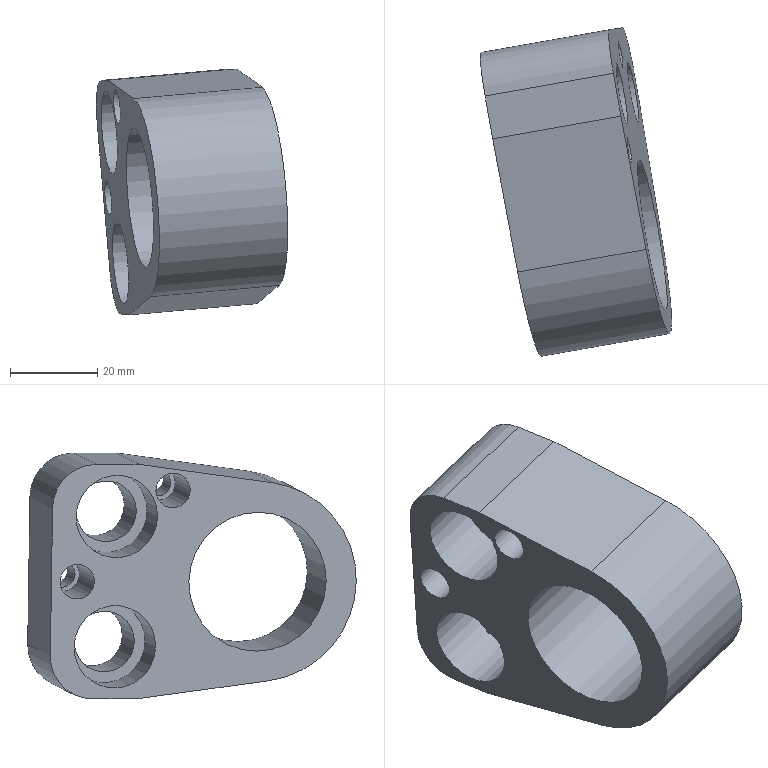Part | NX | features solid 2 | 1 solid | 25 faces | box 43.882 x 75.372 x 56.409 mm | volume 57734 mm3 | cylinder 13 | plane 12 | commonest cylinder face diameters 6 x2 8 x2 14 x2 19 x2 20 x2 32 x1
STEP:
#1=CARTESIAN_POINT('',(1541.538,606.301,14.503));
#2=VERTEX_POINT('',#1);
#3=CARTESIAN_POINT('',(1540.844,610.24,14.503));
#4=DIRECTION('',(0.9811,0.173,0.08716));
#5=DIRECTION('',(0.1736,-0.9848,0.));
#6=AXIS2_PLACEMENT_3D('',#3,#4,#5);
#7=CIRCLE('',#6,4.);
#8=EDGE_CURVE('',#2,#2,#7,.F.);
#9=ORIENTED_EDGE('',*,*,#8,.F.);
#10=EDGE_LOOP('',(#9));
#11=FACE_BOUND('',#10,.T.);
#12=CARTESIAN_POINT('',(1539.47,610.506,29.445));
#13=VERTEX_POINT('',#12);
#14=CARTESIAN_POINT('',(1541.119,601.15,29.445));
#15=DIRECTION('',(-0.9811,-0.173,-0.08716));
#16=DIRECTION('',(-0.1736,0.9848,0.));
#17=AXIS2_PLACEMENT_3D('',#14,#15,#16);
#18=CIRCLE('',#17,9.5);
#19=EDGE_CURVE('',#13,#13,#18,.T.);
#20=ORIENTED_EDGE('',*,*,#19,.F.);
#21=EDGE_LOOP('',(#20));
#22=FACE_BOUND('',#21,.T.);
#23=CARTESIAN_POINT('',(1542.044,610.96,-0.4404));
#24=VERTEX_POINT('',#23);
#25=CARTESIAN_POINT('',(1543.694,601.604,-0.4404));
#26=DIRECTION('',(-0.9811,-0.173,-0.08716));
#27=DIRECTION('',(-0.1736,0.9848,0.));
#28=AXIS2_PLACEMENT_3D('',#25,#26,#27);
#29=CIRCLE('',#28,9.5);
#30=EDGE_CURVE('',#24,#24,#29,.T.);
#31=ORIENTED_EDGE('',*,*,#30,.F.);
#32=EDGE_LOOP('',(#31));
#33=FACE_BOUND('',#32,.T.);
#34=CARTESIAN_POINT('',(1550.915,553.122,14.503));
#35=VERTEX_POINT('',#34);
#36=CARTESIAN_POINT('',(1548.137,568.879,14.503));
#37=DIRECTION('',(0.9811,0.173,0.08716));
#38=DIRECTION('',(0.1736,-0.9848,0.));
#39=AXIS2_PLACEMENT_3D('',#36,#37,#38);
#40=CIRCLE('',#39,16.);
#41=EDGE_CURVE('',#35,#35,#40,.T.);
#42=ORIENTED_EDGE('',*,*,#41,.T.);
#43=EDGE_LOOP('',(#42));
#44=FACE_BOUND('',#43,.T.);
#45=CARTESIAN_POINT('',(1550.629,566.185,-8.203));
#46=VERTEX_POINT('',#45);
#47=CARTESIAN_POINT('',(1545.592,596.862,-12.395));
#48=VERTEX_POINT('',#47);
#49=CARTESIAN_POINT('',(1550.629,566.185,-8.203));
#50=DIRECTION('',(-0.1606,0.9779,-0.1336));
#51=VECTOR('',#50,1000.);
#52=LINE('',#49,#51);
#53=EDGE_CURVE('',#46,#48,#52,.T.);
#54=ORIENTED_EDGE('',*,*,#53,.F.);
#55=CARTESIAN_POINT('',(1546.716,565.495,37.208));
#56=VERTEX_POINT('',#55);
#57=CARTESIAN_POINT('',(1548.137,568.879,14.503));
#58=DIRECTION('',(-0.9811,-0.173,-0.08716));
#59=DIRECTION('',(-0.1736,0.9848,0.));
#60=AXIS2_PLACEMENT_3D('',#57,#58,#59);
#61=CIRCLE('',#60,23.);
#62=EDGE_CURVE('',#46,#56,#61,.T.);
#63=ORIENTED_EDGE('',*,*,#62,.T.);
#64=CARTESIAN_POINT('',(1540.957,596.045,41.4));
#65=VERTEX_POINT('',#64);
#66=CARTESIAN_POINT('',(1546.716,565.495,37.208));
#67=DIRECTION('',(-0.1836,0.9739,0.1336));
#68=VECTOR('',#67,1000.);
#69=LINE('',#66,#68);
#70=EDGE_CURVE('',#56,#65,#69,.T.);
#71=ORIENTED_EDGE('',*,*,#70,.T.);
#72=CARTESIAN_POINT('',(1539.221,605.893,41.4));
#73=VERTEX_POINT('',#72);
#74=CARTESIAN_POINT('',(1540.957,596.045,41.4));
#75=DIRECTION('',(-0.1736,0.9848,0.));
#76=VECTOR('',#75,1000.);
#77=LINE('',#74,#76);
#78=EDGE_CURVE('',#65,#73,#77,.T.);
#79=ORIENTED_EDGE('',*,*,#78,.T.);
#80=CARTESIAN_POINT('',(1538.343,615.892,31.438));
#81=VERTEX_POINT('',#80);
#82=CARTESIAN_POINT('',(1540.079,606.044,31.438));
#83=DIRECTION('',(-0.9811,-0.173,-0.08716));
#84=DIRECTION('',(-0.1736,0.9848,0.));
#85=AXIS2_PLACEMENT_3D('',#82,#83,#84);
#86=CIRCLE('',#85,10.);
#87=EDGE_CURVE('',#73,#81,#86,.T.);
#88=ORIENTED_EDGE('',*,*,#87,.T.);
#89=CARTESIAN_POINT('',(1541.261,616.407,-2.433));
#90=VERTEX_POINT('',#89);
#91=CARTESIAN_POINT('',(1541.261,616.407,-2.433));
#92=DIRECTION('',(-0.08583,-0.01513,0.9962));
#93=VECTOR('',#92,1000.);
#94=LINE('',#91,#93);
#95=EDGE_CURVE('',#90,#81,#94,.T.);
#96=ORIENTED_EDGE('',*,*,#95,.F.);
#97=CARTESIAN_POINT('',(1543.856,606.71,-12.395));
#98=VERTEX_POINT('',#97);
#99=CARTESIAN_POINT('',(1542.998,606.559,-2.433));
#100=DIRECTION('',(-0.9811,-0.173,-0.08716));
#101=DIRECTION('',(-0.1736,0.9848,0.));
#102=AXIS2_PLACEMENT_3D('',#99,#100,#101);
#103=CIRCLE('',#102,10.);
#104=EDGE_CURVE('',#90,#98,#103,.T.);
#105=ORIENTED_EDGE('',*,*,#104,.T.);
#106=CARTESIAN_POINT('',(1545.592,596.862,-12.395));
#107=DIRECTION('',(-0.1736,0.9848,0.));
#108=VECTOR('',#107,1000.);
#109=LINE('',#106,#108);
#110=EDGE_CURVE('',#48,#98,#109,.T.);
#111=ORIENTED_EDGE('',*,*,#110,.F.);
#112=EDGE_LOOP('',(#54,#63,#71,#79,#88,#96,#105,#111));
#113=FACE_BOUND('',#112,.T.);
#114=CARTESIAN_POINT('',(1543.556,584.318,35.423));
#115=VERTEX_POINT('',#114);
#116=CARTESIAN_POINT('',(1542.862,588.257,35.423));
#117=DIRECTION('',(0.9811,0.173,0.08716));
#118=DIRECTION('',(0.1736,-0.9848,0.));
#119=AXIS2_PLACEMENT_3D('',#116,#117,#118);
#120=CIRCLE('',#119,4.);
#121=EDGE_CURVE('',#115,#115,#120,.F.);
#122=ORIENTED_EDGE('',*,*,#121,.F.);
#123=EDGE_LOOP('',(#122));
#124=FACE_BOUND('',#123,.T.);
#125=CARTESIAN_POINT('',(1542.998,606.559,-2.433));
#126=DIRECTION('',(-0.9811,-0.173,-0.08716));
#127=DIRECTION('',(-0.1736,0.9848,0.));
#128=AXIS2_PLACEMENT_3D('',#125,#126,#127);
#129=PLANE('',#128);
#130=ADVANCED_FACE('',(#11,#22,#33,#44,#113,#124),#129,.T.);
#131=CARTESIAN_POINT('',(1569.755,618.385,17.117));
#132=VERTEX_POINT('',#131);
#133=CARTESIAN_POINT('',(1570.276,615.43,17.117));
#134=DIRECTION('',(-0.9811,-0.173,-0.08716));
#135=DIRECTION('',(-0.1736,0.9848,0.));
#136=AXIS2_PLACEMENT_3D('',#133,#134,#135);
#137=CIRCLE('',#136,3.);
#138=EDGE_CURVE('',#132,#132,#137,.T.);
#139=ORIENTED_EDGE('',*,*,#138,.F.);
#140=EDGE_LOOP('',(#139));
#141=FACE_BOUND('',#140,.T.);
#142=CARTESIAN_POINT('',(1559.944,616.655,16.246));
#143=VERTEX_POINT('',#142);
#144=CARTESIAN_POINT('',(1560.465,613.7,16.246));
#145=DIRECTION('',(-0.9811,-0.173,-0.08716));
#146=DIRECTION('',(-0.1736,0.9848,0.));
#147=AXIS2_PLACEMENT_3D('',#144,#145,#146);
#148=CIRCLE('',#147,3.);
#149=EDGE_CURVE('',#143,#143,#148,.T.);
#150=ORIENTED_EDGE('',*,*,#149,.T.);
#151=EDGE_LOOP('',(#150));
#152=FACE_BOUND('',#151,.T.);
#153=CARTESIAN_POINT('',(1540.844,610.24,14.503));
#154=DIRECTION('',(0.9811,0.173,0.08716));
#155=DIRECTION('',(0.1736,-0.9848,0.));
#156=AXIS2_PLACEMENT_3D('',#153,#154,#155);
#157=CYLINDRICAL_SURFACE('',#156,3.);
#158=ADVANCED_FACE('',(#141,#152),#157,.F.);
#159=CARTESIAN_POINT('',(1569.335,613.233,32.06));
#160=VERTEX_POINT('',#159);
#161=CARTESIAN_POINT('',(1570.551,606.34,32.06));
#162=DIRECTION('',(-0.9811,-0.173,-0.08716));
#163=DIRECTION('',(-0.1736,0.9848,0.));
#164=AXIS2_PLACEMENT_3D('',#161,#162,#163);
#165=CIRCLE('',#164,7.);
#166=EDGE_CURVE('',#160,#160,#165,.T.);
#167=ORIENTED_EDGE('',*,*,#166,.F.);
#168=EDGE_LOOP('',(#167));
#169=FACE_BOUND('',#168,.T.);
#170=CARTESIAN_POINT('',(1553.638,610.466,30.666));
#171=VERTEX_POINT('',#170);
#172=CARTESIAN_POINT('',(1554.854,603.572,30.666));
#173=DIRECTION('',(-0.9811,-0.173,-0.08716));
#174=DIRECTION('',(-0.1736,0.9848,0.));
#175=AXIS2_PLACEMENT_3D('',#172,#173,#174);
#176=CIRCLE('',#175,7.);
#177=EDGE_CURVE('',#171,#171,#176,.T.);
#178=ORIENTED_EDGE('',*,*,#177,.T.);
#179=EDGE_LOOP('',(#178));
#180=FACE_BOUND('',#179,.T.);
#181=CARTESIAN_POINT('',(1541.119,601.15,29.445));
#182=DIRECTION('',(0.9811,0.173,0.08716));
#183=DIRECTION('',(0.1736,-0.9848,0.));
#184=AXIS2_PLACEMENT_3D('',#181,#182,#183);
#185=CYLINDRICAL_SURFACE('',#184,7.);
#186=ADVANCED_FACE('',(#169,#180),#185,.F.);
#187=CARTESIAN_POINT('',(1571.91,613.688,2.174));
#188=VERTEX_POINT('',#187);
#189=CARTESIAN_POINT('',(1573.126,606.794,2.174));
#190=DIRECTION('',(-0.9811,-0.173,-0.08716));
#191=DIRECTION('',(-0.1736,0.9848,0.));
#192=AXIS2_PLACEMENT_3D('',#189,#190,#191);
#193=CIRCLE('',#192,7.);
#194=EDGE_CURVE('',#188,#188,#193,.T.);
#195=ORIENTED_EDGE('',*,*,#194,.F.);
#196=EDGE_LOOP('',(#195));
#197=FACE_BOUND('',#196,.T.);
#198=CARTESIAN_POINT('',(1556.213,610.92,0.7798));
#199=VERTEX_POINT('',#198);
#200=CARTESIAN_POINT('',(1557.429,604.026,0.7798));
#201=DIRECTION('',(-0.9811,-0.173,-0.08716));
#202=DIRECTION('',(-0.1736,0.9848,0.));
#203=AXIS2_PLACEMENT_3D('',#200,#201,#202);
#204=CIRCLE('',#203,7.);
#205=EDGE_CURVE('',#199,#199,#204,.T.);
#206=ORIENTED_EDGE('',*,*,#205,.T.);
#207=EDGE_LOOP('',(#206));
#208=FACE_BOUND('',#207,.T.);
#209=CARTESIAN_POINT('',(1543.694,601.604,-0.4404));
#210=DIRECTION('',(0.9811,0.173,0.08716));
#211=DIRECTION('',(0.1736,-0.9848,0.));
#212=AXIS2_PLACEMENT_3D('',#209,#210,#211);
#213=CYLINDRICAL_SURFACE('',#212,7.);
#214=ADVANCED_FACE('',(#197,#208),#213,.F.);
#215=CARTESIAN_POINT('',(1571.772,596.401,38.037));
#216=VERTEX_POINT('',#215);
#217=CARTESIAN_POINT('',(1572.293,593.447,38.037));
#218=DIRECTION('',(-0.9811,-0.173,-0.08716));
#219=DIRECTION('',(-0.1736,0.9848,0.));
#220=AXIS2_PLACEMENT_3D('',#217,#218,#219);
#221=CIRCLE('',#220,3.);
#222=EDGE_CURVE('',#216,#216,#221,.T.);
#223=ORIENTED_EDGE('',*,*,#222,.T.);
#224=EDGE_LOOP('',(#223));
#225=FACE_BOUND('',#224,.T.);
#226=ORIENTED_EDGE('',*,*,#166,.T.);
#227=EDGE_LOOP('',(#226));
#228=FACE_BOUND('',#227,.T.);
#229=CARTESIAN_POINT('',(1580.061,571.375,-5.588));
#230=VERTEX_POINT('',#229);
#231=CARTESIAN_POINT('',(1575.024,602.051,-9.78));
#232=VERTEX_POINT('',#231);
#233=CARTESIAN_POINT('',(1580.061,571.375,-5.588));
#234=DIRECTION('',(-0.1606,0.9779,-0.1336));
#235=VECTOR('',#234,1000.);
#236=LINE('',#233,#235);
#237=EDGE_CURVE('',#230,#232,#236,.T.);
#238=ORIENTED_EDGE('',*,*,#237,.T.);
#239=CARTESIAN_POINT('',(1573.288,611.9,-9.78));
#240=VERTEX_POINT('',#239);
#241=CARTESIAN_POINT('',(1575.024,602.051,-9.78));
#242=DIRECTION('',(-0.1736,0.9848,0.));
#243=VECTOR('',#242,1000.);
#244=LINE('',#241,#243);
#245=EDGE_CURVE('',#232,#240,#244,.T.);
#246=ORIENTED_EDGE('',*,*,#245,.T.);
#247=CARTESIAN_POINT('',(1570.693,621.596,0.1819));
#248=VERTEX_POINT('',#247);
#249=CARTESIAN_POINT('',(1572.429,611.748,0.1819));
#250=DIRECTION('',(-0.9811,-0.173,-0.08716));
#251=DIRECTION('',(-0.1736,0.9848,0.));
#252=AXIS2_PLACEMENT_3D('',#249,#250,#251);
#253=CIRCLE('',#252,10.);
#254=EDGE_CURVE('',#248,#240,#253,.T.);
#255=ORIENTED_EDGE('',*,*,#254,.F.);
#256=CARTESIAN_POINT('',(1567.775,621.082,34.053));
#257=VERTEX_POINT('',#256);
#258=CARTESIAN_POINT('',(1570.693,621.596,0.1819));
#259=DIRECTION('',(-0.08583,-0.01513,0.9962));
#260=VECTOR('',#259,1000.);
#261=LINE('',#258,#260);
#262=EDGE_CURVE('',#248,#257,#261,.T.);
#263=ORIENTED_EDGE('',*,*,#262,.T.);
#264=CARTESIAN_POINT('',(1568.653,611.082,44.014));
#265=VERTEX_POINT('',#264);
#266=CARTESIAN_POINT('',(1569.511,611.234,34.053));
#267=DIRECTION('',(-0.9811,-0.173,-0.08716));
#268=DIRECTION('',(-0.1736,0.9848,0.));
#269=AXIS2_PLACEMENT_3D('',#266,#267,#268);
#270=CIRCLE('',#269,10.);
#271=EDGE_CURVE('',#265,#257,#270,.T.);
#272=ORIENTED_EDGE('',*,*,#271,.F.);
#273=CARTESIAN_POINT('',(1570.389,601.234,44.014));
#274=VERTEX_POINT('',#273);
#275=CARTESIAN_POINT('',(1570.389,601.234,44.014));
#276=DIRECTION('',(-0.1736,0.9848,0.));
#277=VECTOR('',#276,1000.);
#278=LINE('',#275,#277);
#279=EDGE_CURVE('',#274,#265,#278,.T.);
#280=ORIENTED_EDGE('',*,*,#279,.F.);
#281=CARTESIAN_POINT('',(1576.148,570.685,39.823));
#282=VERTEX_POINT('',#281);
#283=CARTESIAN_POINT('',(1576.148,570.685,39.823));
#284=DIRECTION('',(-0.1836,0.9739,0.1336));
#285=VECTOR('',#284,1000.);
#286=LINE('',#283,#285);
#287=EDGE_CURVE('',#282,#274,#286,.T.);
#288=ORIENTED_EDGE('',*,*,#287,.F.);
#289=CARTESIAN_POINT('',(1577.569,574.068,17.117));
#290=DIRECTION('',(-0.9811,-0.173,-0.08716));
#291=DIRECTION('',(-0.1736,0.9848,0.));
#292=AXIS2_PLACEMENT_3D('',#289,#290,#291);
#293=CIRCLE('',#292,23.);
#294=EDGE_CURVE('',#230,#282,#293,.T.);
#295=ORIENTED_EDGE('',*,*,#294,.F.);
#296=EDGE_LOOP('',(#238,#246,#255,#263,#272,#280,#288,#295));
#297=FACE_BOUND('',#296,.T.);
#298=CARTESIAN_POINT('',(1574.487,591.549,17.117));
#299=VERTEX_POINT('',#298);
#300=CARTESIAN_POINT('',(1577.569,574.068,17.117));
#301=DIRECTION('',(-0.9811,-0.173,-0.08716));
#302=DIRECTION('',(-0.1736,0.9848,0.));
#303=AXIS2_PLACEMENT_3D('',#300,#301,#302);
#304=CIRCLE('',#303,17.75);
#305=EDGE_CURVE('',#299,#299,#304,.T.);
#306=ORIENTED_EDGE('',*,*,#305,.T.);
#307=EDGE_LOOP('',(#306));
#308=FACE_BOUND('',#307,.T.);
#309=ORIENTED_EDGE('',*,*,#194,.T.);
#310=EDGE_LOOP('',(#309));
#311=FACE_BOUND('',#310,.T.);
#312=ORIENTED_EDGE('',*,*,#138,.T.);
#313=EDGE_LOOP('',(#312));
#314=FACE_BOUND('',#313,.T.);
#315=CARTESIAN_POINT('',(1572.429,611.748,0.1819));
#316=DIRECTION('',(-0.9811,-0.173,-0.08716));
#317=DIRECTION('',(-0.1736,0.9848,0.));
#318=AXIS2_PLACEMENT_3D('',#315,#316,#317);
#319=PLANE('',#318);
#320=ADVANCED_FACE('',(#225,#228,#297,#308,#311,#314),#319,.F.);
#321=ORIENTED_EDGE('',*,*,#237,.F.);
#322=CARTESIAN_POINT('',(1550.629,566.185,-8.203));
#323=DIRECTION('',(0.9811,0.173,0.08716));
#324=VECTOR('',#323,1000.);
#325=LINE('',#322,#324);
#326=EDGE_CURVE('',#46,#230,#325,.T.);
#327=ORIENTED_EDGE('',*,*,#326,.F.);
#328=ORIENTED_EDGE('',*,*,#53,.T.);
#329=CARTESIAN_POINT('',(1545.592,596.862,-12.395));
#330=DIRECTION('',(0.9811,0.173,0.08716));
#331=VECTOR('',#330,1000.);
#332=LINE('',#329,#331);
#333=EDGE_CURVE('',#48,#232,#332,.T.);
#334=ORIENTED_EDGE('',*,*,#333,.T.);
#335=EDGE_LOOP('',(#321,#327,#328,#334));
#336=FACE_BOUND('',#335,.T.);
#337=CARTESIAN_POINT('',(1550.629,566.185,-8.203));
#338=DIRECTION('',(0.1083,-0.1171,-0.9872));
#339=DIRECTION('',(-0.1606,0.9779,-0.1336));
#340=AXIS2_PLACEMENT_3D('',#337,#338,#339);
#341=PLANE('',#340);
#342=ADVANCED_FACE('',(#336),#341,.T.);
#343=ORIENTED_EDGE('',*,*,#245,.F.);
#344=ORIENTED_EDGE('',*,*,#333,.F.);
#345=ORIENTED_EDGE('',*,*,#110,.T.);
#346=CARTESIAN_POINT('',(1543.856,606.71,-12.395));
#347=DIRECTION('',(0.9811,0.173,0.08716));
#348=VECTOR('',#347,1000.);
#349=LINE('',#346,#348);
#350=EDGE_CURVE('',#98,#240,#349,.T.);
#351=ORIENTED_EDGE('',*,*,#350,.T.);
#352=EDGE_LOOP('',(#343,#344,#345,#351));
#353=FACE_BOUND('',#352,.T.);
#354=CARTESIAN_POINT('',(1545.592,596.862,-12.395));
#355=DIRECTION('',(0.08583,0.01513,-0.9962));
#356=DIRECTION('',(-0.1736,0.9848,0.));
#357=AXIS2_PLACEMENT_3D('',#354,#355,#356);
#358=PLANE('',#357);
#359=ADVANCED_FACE('',(#353),#358,.T.);
#360=ORIENTED_EDGE('',*,*,#254,.T.);
#361=ORIENTED_EDGE('',*,*,#350,.F.);
#362=ORIENTED_EDGE('',*,*,#104,.F.);
#363=CARTESIAN_POINT('',(1541.261,616.407,-2.433));
#364=DIRECTION('',(0.9811,0.173,0.08716));
#365=VECTOR('',#364,1000.);
#366=LINE('',#363,#365);
#367=EDGE_CURVE('',#90,#248,#366,.T.);
#368=ORIENTED_EDGE('',*,*,#367,.T.);
#369=EDGE_LOOP('',(#360,#361,#362,#368));
#370=FACE_BOUND('',#369,.T.);
#371=CARTESIAN_POINT('',(1542.998,606.559,-2.433));
#372=DIRECTION('',(0.9811,0.173,0.08716));
#373=DIRECTION('',(0.1736,-0.9848,0.));
#374=AXIS2_PLACEMENT_3D('',#371,#372,#373);
#375=CYLINDRICAL_SURFACE('',#374,10.);
#376=ADVANCED_FACE('',(#370),#375,.T.);
#377=ORIENTED_EDGE('',*,*,#262,.F.);
#378=ORIENTED_EDGE('',*,*,#367,.F.);
#379=ORIENTED_EDGE('',*,*,#95,.T.);
#380=CARTESIAN_POINT('',(1538.343,615.892,31.438));
#381=DIRECTION('',(0.9811,0.173,0.08716));
#382=VECTOR('',#381,1000.);
#383=LINE('',#380,#382);
#384=EDGE_CURVE('',#81,#257,#383,.T.);
#385=ORIENTED_EDGE('',*,*,#384,.T.);
#386=EDGE_LOOP('',(#377,#378,#379,#385));
#387=FACE_BOUND('',#386,.T.);
#388=CARTESIAN_POINT('',(1541.261,616.407,-2.433));
#389=DIRECTION('',(-0.1736,0.9848,0.));
#390=DIRECTION('',(-0.08583,-0.01513,0.9962));
#391=AXIS2_PLACEMENT_3D('',#388,#389,#390);
#392=PLANE('',#391);
#393=ADVANCED_FACE('',(#387),#392,.T.);
#394=ORIENTED_EDGE('',*,*,#271,.T.);
#395=ORIENTED_EDGE('',*,*,#384,.F.);
#396=ORIENTED_EDGE('',*,*,#87,.F.);
#397=CARTESIAN_POINT('',(1539.221,605.893,41.4));
#398=DIRECTION('',(0.9811,0.173,0.08716));
#399=VECTOR('',#398,1000.);
#400=LINE('',#397,#399);
#401=EDGE_CURVE('',#73,#265,#400,.T.);
#402=ORIENTED_EDGE('',*,*,#401,.T.);
#403=EDGE_LOOP('',(#394,#395,#396,#402));
#404=FACE_BOUND('',#403,.T.);
#405=CARTESIAN_POINT('',(1540.079,606.044,31.438));
#406=DIRECTION('',(0.9811,0.173,0.08716));
#407=DIRECTION('',(0.1736,-0.9848,0.));
#408=AXIS2_PLACEMENT_3D('',#405,#406,#407);
#409=CYLINDRICAL_SURFACE('',#408,10.);
#410=ADVANCED_FACE('',(#404),#409,.T.);
#411=ORIENTED_EDGE('',*,*,#279,.T.);
#412=ORIENTED_EDGE('',*,*,#401,.F.);
#413=ORIENTED_EDGE('',*,*,#78,.F.);
#414=CARTESIAN_POINT('',(1540.957,596.045,41.4));
#415=DIRECTION('',(0.9811,0.173,0.08716));
#416=VECTOR('',#415,1000.);
#417=LINE('',#414,#416);
#418=EDGE_CURVE('',#65,#274,#417,.T.);
#419=ORIENTED_EDGE('',*,*,#418,.T.);
#420=EDGE_LOOP('',(#411,#412,#413,#419));
#421=FACE_BOUND('',#420,.T.);
#422=CARTESIAN_POINT('',(1540.957,596.045,41.4));
#423=DIRECTION('',(0.08583,0.01513,-0.9962));
#424=DIRECTION('',(-0.1736,0.9848,0.));
#425=AXIS2_PLACEMENT_3D('',#422,#423,#424);
#426=PLANE('',#425);
#427=ADVANCED_FACE('',(#421),#426,.F.);
#428=ORIENTED_EDGE('',*,*,#287,.T.);
#429=ORIENTED_EDGE('',*,*,#418,.F.);
#430=ORIENTED_EDGE('',*,*,#70,.F.);
#431=CARTESIAN_POINT('',(1546.716,565.495,37.208));
#432=DIRECTION('',(0.9811,0.173,0.08716));
#433=VECTOR('',#432,1000.);
#434=LINE('',#431,#433);
#435=EDGE_CURVE('',#56,#282,#434,.T.);
#436=ORIENTED_EDGE('',*,*,#435,.T.);
#437=EDGE_LOOP('',(#428,#429,#430,#436));
#438=FACE_BOUND('',#437,.T.);
#439=CARTESIAN_POINT('',(1546.716,565.495,37.208));
#440=DIRECTION('',(0.06176,0.1471,-0.9872));
#441=DIRECTION('',(-0.1836,0.9739,0.1336));
#442=AXIS2_PLACEMENT_3D('',#439,#440,#441);
#443=PLANE('',#442);
#444=ADVANCED_FACE('',(#438),#443,.F.);
#445=ORIENTED_EDGE('',*,*,#294,.T.);
#446=ORIENTED_EDGE('',*,*,#435,.F.);
#447=ORIENTED_EDGE('',*,*,#62,.F.);
#448=ORIENTED_EDGE('',*,*,#326,.T.);
#449=EDGE_LOOP('',(#445,#446,#447,#448));
#450=FACE_BOUND('',#449,.T.);
#451=CARTESIAN_POINT('',(1548.137,568.879,14.503));
#452=DIRECTION('',(0.9811,0.173,0.08716));
#453=DIRECTION('',(0.1736,-0.9848,0.));
#454=AXIS2_PLACEMENT_3D('',#451,#452,#453);
#455=CYLINDRICAL_SURFACE('',#454,23.);
#456=ADVANCED_FACE('',(#450),#455,.T.);
#457=CARTESIAN_POINT('',(1569.885,588.96,16.681));
#458=VERTEX_POINT('',#457);
#459=CARTESIAN_POINT('',(1572.664,573.203,16.681));
#460=DIRECTION('',(-0.9811,-0.173,-0.08716));
#461=DIRECTION('',(-0.1736,0.9848,0.));
#462=AXIS2_PLACEMENT_3D('',#459,#460,#461);
#463=CIRCLE('',#462,16.);
#464=EDGE_CURVE('',#458,#458,#463,.F.);
#465=ORIENTED_EDGE('',*,*,#464,.T.);
#466=EDGE_LOOP('',(#465));
#467=FACE_BOUND('',#466,.T.);
#468=ORIENTED_EDGE('',*,*,#41,.F.);
#469=EDGE_LOOP('',(#468));
#470=FACE_BOUND('',#469,.T.);
#471=CARTESIAN_POINT('',(1548.137,568.879,14.503));
#472=DIRECTION('',(0.9811,0.173,0.08716));
#473=DIRECTION('',(0.1736,-0.9848,0.));
#474=AXIS2_PLACEMENT_3D('',#471,#472,#473);
#475=CYLINDRICAL_SURFACE('',#474,16.);
#476=ADVANCED_FACE('',(#467,#470),#475,.F.);
#477=CARTESIAN_POINT('',(1569.581,590.684,16.681));
#478=VERTEX_POINT('',#477);
#479=CARTESIAN_POINT('',(1572.664,573.203,16.681));
#480=DIRECTION('',(-0.9811,-0.173,-0.08716));
#481=DIRECTION('',(-0.1736,0.9848,0.));
#482=AXIS2_PLACEMENT_3D('',#479,#480,#481);
#483=CIRCLE('',#482,17.75);
#484=EDGE_CURVE('',#478,#478,#483,.T.);
#485=ORIENTED_EDGE('',*,*,#484,.F.);
#486=EDGE_LOOP('',(#485));
#487=FACE_BOUND('',#486,.T.);
#488=ORIENTED_EDGE('',*,*,#464,.F.);
#489=EDGE_LOOP('',(#488));
#490=FACE_BOUND('',#489,.T.);
#491=CARTESIAN_POINT('',(1572.664,573.203,16.681));
#492=DIRECTION('',(-0.9811,-0.173,-0.08716));
#493=DIRECTION('',(-0.1736,0.9848,0.));
#494=AXIS2_PLACEMENT_3D('',#491,#492,#493);
#495=PLANE('',#494);
#496=ADVANCED_FACE('',(#487,#490),#495,.F.);
#497=ORIENTED_EDGE('',*,*,#484,.T.);
#498=EDGE_LOOP('',(#497));
#499=FACE_BOUND('',#498,.T.);
#500=ORIENTED_EDGE('',*,*,#305,.F.);
#501=EDGE_LOOP('',(#500));
#502=FACE_BOUND('',#501,.T.);
#503=CARTESIAN_POINT('',(1572.664,573.203,16.681));
#504=DIRECTION('',(0.9811,0.173,0.08716));
#505=DIRECTION('',(0.1736,-0.9848,0.));
#506=AXIS2_PLACEMENT_3D('',#503,#504,#505);
#507=CYLINDRICAL_SURFACE('',#506,17.75);
#508=ADVANCED_FACE('',(#499,#502),#507,.F.);
#509=CARTESIAN_POINT('',(1561.962,594.671,37.166));
#510=VERTEX_POINT('',#509);
#511=CARTESIAN_POINT('',(1562.483,591.717,37.166));
#512=DIRECTION('',(-0.9811,-0.173,-0.08716));
#513=DIRECTION('',(-0.1736,0.9848,0.));
#514=AXIS2_PLACEMENT_3D('',#511,#512,#513);
#515=CIRCLE('',#514,3.);
#516=EDGE_CURVE('',#510,#510,#515,.T.);
#517=ORIENTED_EDGE('',*,*,#516,.T.);
#518=EDGE_LOOP('',(#517));
#519=FACE_BOUND('',#518,.T.);
#520=ORIENTED_EDGE('',*,*,#222,.F.);
#521=EDGE_LOOP('',(#520));
#522=FACE_BOUND('',#521,.T.);
#523=CARTESIAN_POINT('',(1542.862,588.257,35.423));
#524=DIRECTION('',(0.9811,0.173,0.08716));
#525=DIRECTION('',(0.1736,-0.9848,0.));
#526=AXIS2_PLACEMENT_3D('',#523,#524,#525);
#527=CYLINDRICAL_SURFACE('',#526,3.);
#528=ADVANCED_FACE('',(#519,#522),#527,.F.);
#529=CARTESIAN_POINT('',(1555.779,613.382,0.7798));
#530=VERTEX_POINT('',#529);
#531=CARTESIAN_POINT('',(1557.429,604.026,0.7798));
#532=DIRECTION('',(-0.9811,-0.173,-0.08716));
#533=DIRECTION('',(-0.1736,0.9848,0.));
#534=AXIS2_PLACEMENT_3D('',#531,#532,#533);
#535=CIRCLE('',#534,9.5);
#536=EDGE_CURVE('',#530,#530,#535,.T.);
#537=ORIENTED_EDGE('',*,*,#536,.F.);
#538=EDGE_LOOP('',(#537));
#539=FACE_BOUND('',#538,.T.);
#540=ORIENTED_EDGE('',*,*,#30,.T.);
#541=EDGE_LOOP('',(#540));
#542=FACE_BOUND('',#541,.T.);
#543=CARTESIAN_POINT('',(1557.429,604.026,0.7798));
#544=DIRECTION('',(-0.9811,-0.173,-0.08716));
#545=DIRECTION('',(-0.1736,0.9848,0.));
#546=AXIS2_PLACEMENT_3D('',#543,#544,#545);
#547=CYLINDRICAL_SURFACE('',#546,9.5);
#548=ADVANCED_FACE('',(#539,#542),#547,.F.);
#549=ORIENTED_EDGE('',*,*,#205,.F.);
#550=EDGE_LOOP('',(#549));
#551=FACE_BOUND('',#550,.T.);
#552=ORIENTED_EDGE('',*,*,#536,.T.);
#553=EDGE_LOOP('',(#552));
#554=FACE_BOUND('',#553,.T.);
#555=CARTESIAN_POINT('',(1557.429,604.026,0.7798));
#556=DIRECTION('',(-0.9811,-0.173,-0.08716));
#557=DIRECTION('',(-0.1736,0.9848,0.));
#558=AXIS2_PLACEMENT_3D('',#555,#556,#557);
#559=PLANE('',#558);
#560=ADVANCED_FACE('',(#551,#554),#559,.T.);
#561=CARTESIAN_POINT('',(1553.204,612.928,30.666));
#562=VERTEX_POINT('',#561);
#563=CARTESIAN_POINT('',(1554.854,603.572,30.666));
#564=DIRECTION('',(-0.9811,-0.173,-0.08716));
#565=DIRECTION('',(-0.1736,0.9848,0.));
#566=AXIS2_PLACEMENT_3D('',#563,#564,#565);
#567=CIRCLE('',#566,9.5);
#568=EDGE_CURVE('',#562,#562,#567,.T.);
#569=ORIENTED_EDGE('',*,*,#568,.F.);
#570=EDGE_LOOP('',(#569));
#571=FACE_BOUND('',#570,.T.);
#572=ORIENTED_EDGE('',*,*,#19,.T.);
#573=EDGE_LOOP('',(#572));
#574=FACE_BOUND('',#573,.T.);
#575=CARTESIAN_POINT('',(1554.854,603.572,30.666));
#576=DIRECTION('',(-0.9811,-0.173,-0.08716));
#577=DIRECTION('',(-0.1736,0.9848,0.));
#578=AXIS2_PLACEMENT_3D('',#575,#576,#577);
#579=CYLINDRICAL_SURFACE('',#578,9.5);
#580=ADVANCED_FACE('',(#571,#574),#579,.F.);
#581=ORIENTED_EDGE('',*,*,#177,.F.);
#582=EDGE_LOOP('',(#581));
#583=FACE_BOUND('',#582,.T.);
#584=ORIENTED_EDGE('',*,*,#568,.T.);
#585=EDGE_LOOP('',(#584));
#586=FACE_BOUND('',#585,.T.);
#587=CARTESIAN_POINT('',(1554.854,603.572,30.666));
#588=DIRECTION('',(-0.9811,-0.173,-0.08716));
#589=DIRECTION('',(-0.1736,0.9848,0.));
#590=AXIS2_PLACEMENT_3D('',#587,#588,#589);
#591=PLANE('',#590);
#592=ADVANCED_FACE('',(#583,#586),#591,.T.);
#593=ORIENTED_EDGE('',*,*,#149,.F.);
#594=EDGE_LOOP('',(#593));
#595=FACE_BOUND('',#594,.T.);
#596=CARTESIAN_POINT('',(1561.16,609.761,16.246));
#597=VERTEX_POINT('',#596);
#598=CARTESIAN_POINT('',(1560.465,613.7,16.246));
#599=DIRECTION('',(0.9811,0.173,0.08716));
#600=DIRECTION('',(0.1736,-0.9848,0.));
#601=AXIS2_PLACEMENT_3D('',#598,#599,#600);
#602=CIRCLE('',#601,4.);
#603=EDGE_CURVE('',#597,#597,#602,.F.);
#604=ORIENTED_EDGE('',*,*,#603,.T.);
#605=EDGE_LOOP('',(#604));
#606=FACE_BOUND('',#605,.T.);
#607=CARTESIAN_POINT('',(1560.465,613.7,16.246));
#608=DIRECTION('',(0.9811,0.173,0.08716));
#609=DIRECTION('',(0.1736,-0.9848,0.));
#610=AXIS2_PLACEMENT_3D('',#607,#608,#609);
#611=PLANE('',#610);
#612=ADVANCED_FACE('',(#595,#606),#611,.F.);
#613=ORIENTED_EDGE('',*,*,#603,.F.);
#614=EDGE_LOOP('',(#613));
#615=FACE_BOUND('',#614,.T.);
#616=ORIENTED_EDGE('',*,*,#8,.T.);
#617=EDGE_LOOP('',(#616));
#618=FACE_BOUND('',#617,.T.);
#619=CARTESIAN_POINT('',(1540.844,610.24,14.503));
#620=DIRECTION('',(0.9811,0.173,0.08716));
#621=DIRECTION('',(0.1736,-0.9848,0.));
#622=AXIS2_PLACEMENT_3D('',#619,#620,#621);
#623=CYLINDRICAL_SURFACE('',#622,4.);
#624=ADVANCED_FACE('',(#615,#618),#623,.F.);
#625=ORIENTED_EDGE('',*,*,#516,.F.);
#626=EDGE_LOOP('',(#625));
#627=FACE_BOUND('',#626,.T.);
#628=CARTESIAN_POINT('',(1563.177,587.777,37.166));
#629=VERTEX_POINT('',#628);
#630=CARTESIAN_POINT('',(1562.483,591.717,37.166));
#631=DIRECTION('',(0.9811,0.173,0.08716));
#632=DIRECTION('',(0.1736,-0.9848,0.));
#633=AXIS2_PLACEMENT_3D('',#630,#631,#632);
#634=CIRCLE('',#633,4.);
#635=EDGE_CURVE('',#629,#629,#634,.F.);
#636=ORIENTED_EDGE('',*,*,#635,.T.);
#637=EDGE_LOOP('',(#636));
#638=FACE_BOUND('',#637,.T.);
#639=CARTESIAN_POINT('',(1562.483,591.717,37.166));
#640=DIRECTION('',(0.9811,0.173,0.08716));
#641=DIRECTION('',(0.1736,-0.9848,0.));
#642=AXIS2_PLACEMENT_3D('',#639,#640,#641);
#643=PLANE('',#642);
#644=ADVANCED_FACE('',(#627,#638),#643,.F.);
#645=ORIENTED_EDGE('',*,*,#635,.F.);
#646=EDGE_LOOP('',(#645));
#647=FACE_BOUND('',#646,.T.);
#648=ORIENTED_EDGE('',*,*,#121,.T.);
#649=EDGE_LOOP('',(#648));
#650=FACE_BOUND('',#649,.T.);
#651=CARTESIAN_POINT('',(1542.862,588.257,35.423));
#652=DIRECTION('',(0.9811,0.173,0.08716));
#653=DIRECTION('',(0.1736,-0.9848,0.));
#654=AXIS2_PLACEMENT_3D('',#651,#652,#653);
#655=CYLINDRICAL_SURFACE('',#654,4.);
#656=ADVANCED_FACE('',(#647,#650),#655,.F.);
#657=CLOSED_SHELL('',(#130,#158,#186,#214,#320,#342,#359,#376,#393,#410,#427,#444,#456,#476,#496,#508,#528,#548,#560,#580,#592,#612,#624,#644,#656));
#658=MANIFOLD_SOLID_BREP('',#657);
#659=(LENGTH_UNIT()NAMED_UNIT(*)SI_UNIT(.MILLI.,.METRE.));
#660=UNCERTAINTY_MEASURE_WITH_UNIT(LENGTH_MEASURE(0.00001),#659,'','');
#661=(NAMED_UNIT(*)PLANE_ANGLE_UNIT()SI_UNIT($,.RADIAN.));
#662=(NAMED_UNIT(*)SI_UNIT($,.STERADIAN.)SOLID_ANGLE_UNIT());
#663=(GEOMETRIC_REPRESENTATION_CONTEXT(3)GLOBAL_UNCERTAINTY_ASSIGNED_CONTEXT((#660))GLOBAL_UNIT_ASSIGNED_CONTEXT((#659,#661,#662))REPRESENTATION_CONTEXT('',''));
#664=ADVANCED_BREP_SHAPE_REPRESENTATION('',(#658),#663);